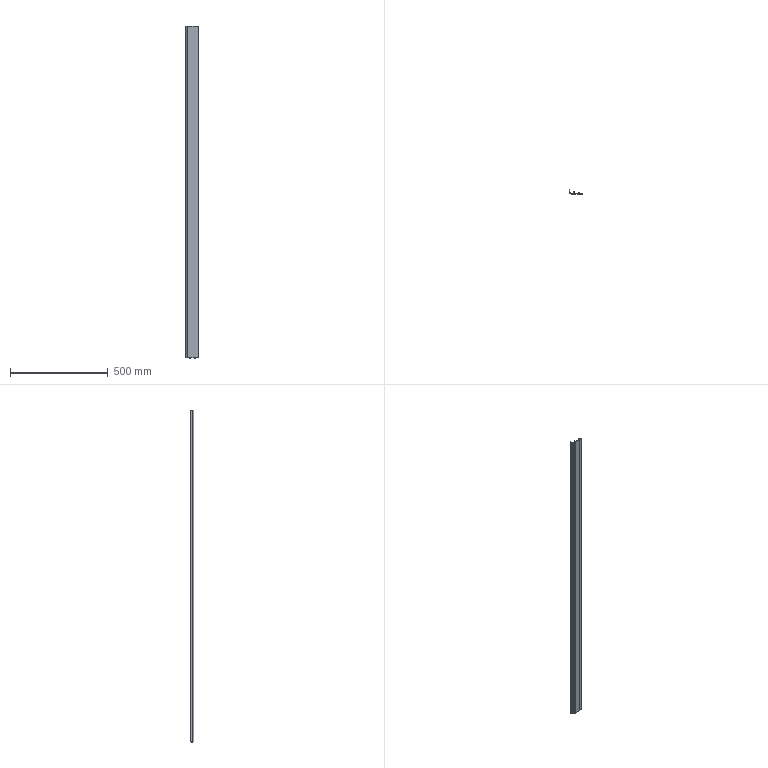Part | STEP file | 51E-01201JG10 | 1 solid | 49 faces | box 67.801 x 18.48 x 1700 mm | volume 194300 mm3 | cylinder 28 | plane 21 | commonest cylinder face diameters 0.4 x11 0.6 x3 1 x3 1.2 x2 1.4 x2 4 x2